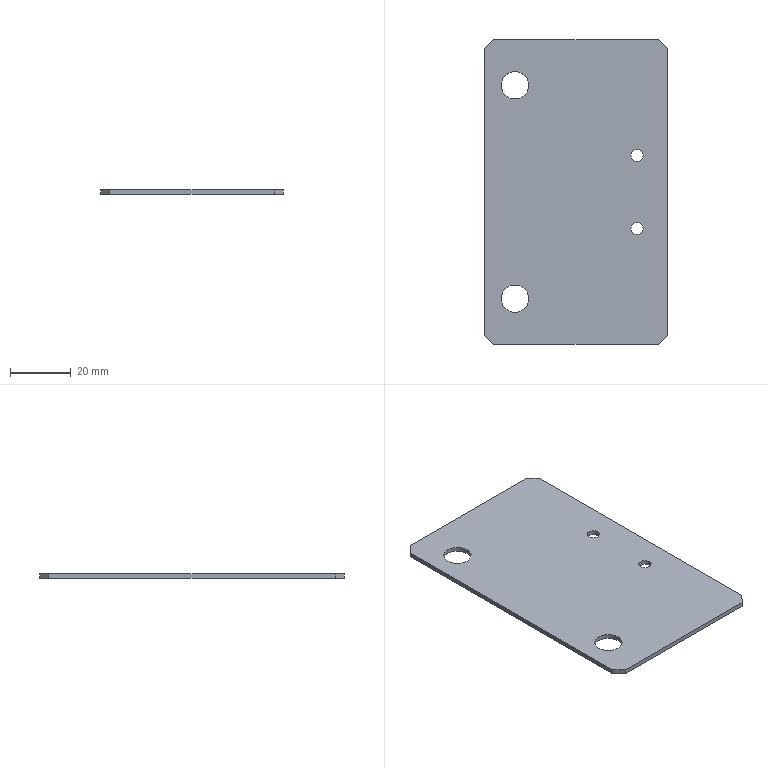Part | STEP file | 1 solid | 18 faces | box 60 x 100 x 1.5 mm | volume 8744 mm3 | plane 10 | cylinder 8 | commonest cylinder face diameters 4 x4 9 x4
STEP:
#1=CARTESIAN_POINT('',(0.,0.,0.));
#2=DIRECTION('',(0.,0.,1.));
#3=DIRECTION('',(1.,0.,0.));
#4=AXIS2_PLACEMENT_3D('',#1,#2,#3);
#5=CARTESIAN_POINT('',(-15.5,-35.,-1.5));
#6=VERTEX_POINT('',#5);
#7=CARTESIAN_POINT('',(-15.5,-35.,0.));
#8=VERTEX_POINT('',#7);
#9=CARTESIAN_POINT('',(-15.5,-35.,-1.5));
#10=DIRECTION('',(0.,0.,1.));
#11=VECTOR('',#10,1.);
#12=LINE('',#9,#11);
#13=CARTESIAN_POINT('',(-20.,-35.,-1.5));
#14=DIRECTION('',(0.,0.,1.));
#15=DIRECTION('',(1.,0.,0.));
#16=AXIS2_PLACEMENT_3D('',#13,#14,#15);
#17=CYLINDRICAL_SURFACE('',#16,4.5);
#18=CARTESIAN_POINT('',(6.283,0.));
#19=DIRECTION('',(0.,1.));
#20=VECTOR('',#19,1.);
#21=LINE('',#18,#20);
#22=(GEOMETRIC_REPRESENTATION_CONTEXT(2)PARAMETRIC_REPRESENTATION_CONTEXT()REPRESENTATION_CONTEXT('',''));
#23=DEFINITIONAL_REPRESENTATION('',(#21),#22);
#24=PCURVE('',#17,#23);
#25=CARTESIAN_POINT('',(-20.,-35.,-1.5));
#26=DIRECTION('',(0.,0.,1.));
#27=DIRECTION('',(1.,0.,0.));
#28=AXIS2_PLACEMENT_3D('',#25,#26,#27);
#29=CYLINDRICAL_SURFACE('',#28,4.5);
#30=CARTESIAN_POINT('',(0.,0.));
#31=DIRECTION('',(0.,1.));
#32=VECTOR('',#31,1.);
#33=LINE('',#30,#32);
#34=(GEOMETRIC_REPRESENTATION_CONTEXT(2)PARAMETRIC_REPRESENTATION_CONTEXT()REPRESENTATION_CONTEXT('',''));
#35=DEFINITIONAL_REPRESENTATION('',(#33),#34);
#36=PCURVE('',#29,#35);
#37=SURFACE_CURVE('',#12,(#24,#36),.PCURVE_S1.);
#38=EDGE_CURVE('',#6,#8,#37,.T.);
#39=ORIENTED_EDGE('',*,*,#38,.T.);
#40=CARTESIAN_POINT('',(-24.5,-35.,0.));
#41=VERTEX_POINT('',#40);
#42=CARTESIAN_POINT('',(-20.,-35.,0.));
#43=DIRECTION('',(0.,0.,1.));
#44=DIRECTION('',(1.,0.,0.));
#45=AXIS2_PLACEMENT_3D('',#42,#43,#44);
#46=CIRCLE('',#45,4.5);
#47=CARTESIAN_POINT('',(0.,1.5));
#48=DIRECTION('',(1.,0.));
#49=VECTOR('',#48,1.);
#50=LINE('',#47,#49);
#51=(GEOMETRIC_REPRESENTATION_CONTEXT(2)PARAMETRIC_REPRESENTATION_CONTEXT()REPRESENTATION_CONTEXT('',''));
#52=DEFINITIONAL_REPRESENTATION('',(#50),#51);
#53=PCURVE('',#17,#52);
#54=CARTESIAN_POINT('',(0.,0.,0.));
#55=DIRECTION('',(0.,0.,1.));
#56=DIRECTION('',(1.,0.,0.));
#57=AXIS2_PLACEMENT_3D('',#54,#55,#56);
#58=PLANE('',#57);
#59=CARTESIAN_POINT('',(-20.,-35.));
#60=DIRECTION('',(1.,0.));
#61=AXIS2_PLACEMENT_2D('',#59,#60);
#62=CIRCLE('',#61,4.5);
#63=(GEOMETRIC_REPRESENTATION_CONTEXT(2)PARAMETRIC_REPRESENTATION_CONTEXT()REPRESENTATION_CONTEXT('',''));
#64=DEFINITIONAL_REPRESENTATION('',(#62),#63);
#65=PCURVE('',#58,#64);
#66=SURFACE_CURVE('',#46,(#53,#65),.PCURVE_S1.);
#67=EDGE_CURVE('',#41,#8,#66,.T.);
#68=ORIENTED_EDGE('',*,*,#67,.F.);
#69=CARTESIAN_POINT('',(-24.5,-35.,-1.5));
#70=VERTEX_POINT('',#69);
#71=CARTESIAN_POINT('',(-24.5,-35.,-1.5));
#72=DIRECTION('',(0.,0.,1.));
#73=VECTOR('',#72,1.);
#74=LINE('',#71,#73);
#75=CARTESIAN_POINT('',(3.142,0.));
#76=DIRECTION('',(0.,1.));
#77=VECTOR('',#76,1.);
#78=LINE('',#75,#77);
#79=(GEOMETRIC_REPRESENTATION_CONTEXT(2)PARAMETRIC_REPRESENTATION_CONTEXT()REPRESENTATION_CONTEXT('',''));
#80=DEFINITIONAL_REPRESENTATION('',(#78),#79);
#81=PCURVE('',#17,#80);
#82=CARTESIAN_POINT('',(3.142,0.));
#83=DIRECTION('',(0.,1.));
#84=VECTOR('',#83,1.);
#85=LINE('',#82,#84);
#86=(GEOMETRIC_REPRESENTATION_CONTEXT(2)PARAMETRIC_REPRESENTATION_CONTEXT()REPRESENTATION_CONTEXT('',''));
#87=DEFINITIONAL_REPRESENTATION('',(#85),#86);
#88=PCURVE('',#29,#87);
#89=SURFACE_CURVE('',#74,(#81,#88),.PCURVE_S1.);
#90=EDGE_CURVE('',#70,#41,#89,.T.);
#91=ORIENTED_EDGE('',*,*,#90,.F.);
#92=CARTESIAN_POINT('',(-20.,-35.,-1.5));
#93=DIRECTION('',(0.,0.,1.));
#94=DIRECTION('',(1.,0.,0.));
#95=AXIS2_PLACEMENT_3D('',#92,#93,#94);
#96=CIRCLE('',#95,4.5);
#97=CARTESIAN_POINT('',(0.,0.));
#98=DIRECTION('',(1.,0.));
#99=VECTOR('',#98,1.);
#100=LINE('',#97,#99);
#101=(GEOMETRIC_REPRESENTATION_CONTEXT(2)PARAMETRIC_REPRESENTATION_CONTEXT()REPRESENTATION_CONTEXT('',''));
#102=DEFINITIONAL_REPRESENTATION('',(#100),#101);
#103=PCURVE('',#17,#102);
#104=CARTESIAN_POINT('',(0.,0.,-1.5));
#105=DIRECTION('',(0.,0.,1.));
#106=DIRECTION('',(1.,0.,0.));
#107=AXIS2_PLACEMENT_3D('',#104,#105,#106);
#108=PLANE('',#107);
#109=CARTESIAN_POINT('',(-20.,-35.));
#110=DIRECTION('',(1.,0.));
#111=AXIS2_PLACEMENT_2D('',#109,#110);
#112=CIRCLE('',#111,4.5);
#113=(GEOMETRIC_REPRESENTATION_CONTEXT(2)PARAMETRIC_REPRESENTATION_CONTEXT()REPRESENTATION_CONTEXT('',''));
#114=DEFINITIONAL_REPRESENTATION('',(#112),#113);
#115=PCURVE('',#108,#114);
#116=SURFACE_CURVE('',#96,(#103,#115),.PCURVE_S1.);
#117=EDGE_CURVE('',#70,#6,#116,.T.);
#118=ORIENTED_EDGE('',*,*,#117,.T.);
#119=EDGE_LOOP('',(#39,#68,#91,#118));
#120=FACE_BOUND('',#119,.F.);
#121=ADVANCED_FACE('',(#120),#17,.F.);
#122=CARTESIAN_POINT('',(-15.5,35.,-1.5));
#123=VERTEX_POINT('',#122);
#124=CARTESIAN_POINT('',(-15.5,35.,0.));
#125=VERTEX_POINT('',#124);
#126=CARTESIAN_POINT('',(-15.5,35.,-1.5));
#127=DIRECTION('',(0.,0.,1.));
#128=VECTOR('',#127,1.);
#129=LINE('',#126,#128);
#130=CARTESIAN_POINT('',(-20.,35.,-1.5));
#131=DIRECTION('',(0.,0.,1.));
#132=DIRECTION('',(1.,0.,0.));
#133=AXIS2_PLACEMENT_3D('',#130,#131,#132);
#134=CYLINDRICAL_SURFACE('',#133,4.5);
#135=CARTESIAN_POINT('',(6.283,0.));
#136=DIRECTION('',(0.,1.));
#137=VECTOR('',#136,1.);
#138=LINE('',#135,#137);
#139=(GEOMETRIC_REPRESENTATION_CONTEXT(2)PARAMETRIC_REPRESENTATION_CONTEXT()REPRESENTATION_CONTEXT('',''));
#140=DEFINITIONAL_REPRESENTATION('',(#138),#139);
#141=PCURVE('',#134,#140);
#142=CARTESIAN_POINT('',(-20.,35.,-1.5));
#143=DIRECTION('',(0.,0.,1.));
#144=DIRECTION('',(1.,0.,0.));
#145=AXIS2_PLACEMENT_3D('',#142,#143,#144);
#146=CYLINDRICAL_SURFACE('',#145,4.5);
#147=CARTESIAN_POINT('',(0.,0.));
#148=DIRECTION('',(0.,1.));
#149=VECTOR('',#148,1.);
#150=LINE('',#147,#149);
#151=(GEOMETRIC_REPRESENTATION_CONTEXT(2)PARAMETRIC_REPRESENTATION_CONTEXT()REPRESENTATION_CONTEXT('',''));
#152=DEFINITIONAL_REPRESENTATION('',(#150),#151);
#153=PCURVE('',#146,#152);
#154=SURFACE_CURVE('',#129,(#141,#153),.PCURVE_S1.);
#155=EDGE_CURVE('',#123,#125,#154,.T.);
#156=ORIENTED_EDGE('',*,*,#155,.T.);
#157=CARTESIAN_POINT('',(-24.5,35.,0.));
#158=VERTEX_POINT('',#157);
#159=CARTESIAN_POINT('',(-20.,35.,0.));
#160=DIRECTION('',(0.,0.,1.));
#161=DIRECTION('',(1.,0.,0.));
#162=AXIS2_PLACEMENT_3D('',#159,#160,#161);
#163=CIRCLE('',#162,4.5);
#164=CARTESIAN_POINT('',(0.,1.5));
#165=DIRECTION('',(1.,0.));
#166=VECTOR('',#165,1.);
#167=LINE('',#164,#166);
#168=(GEOMETRIC_REPRESENTATION_CONTEXT(2)PARAMETRIC_REPRESENTATION_CONTEXT()REPRESENTATION_CONTEXT('',''));
#169=DEFINITIONAL_REPRESENTATION('',(#167),#168);
#170=PCURVE('',#134,#169);
#171=CARTESIAN_POINT('',(-20.,35.));
#172=DIRECTION('',(1.,0.));
#173=AXIS2_PLACEMENT_2D('',#171,#172);
#174=CIRCLE('',#173,4.5);
#175=(GEOMETRIC_REPRESENTATION_CONTEXT(2)PARAMETRIC_REPRESENTATION_CONTEXT()REPRESENTATION_CONTEXT('',''));
#176=DEFINITIONAL_REPRESENTATION('',(#174),#175);
#177=PCURVE('',#58,#176);
#178=SURFACE_CURVE('',#163,(#170,#177),.PCURVE_S1.);
#179=EDGE_CURVE('',#158,#125,#178,.T.);
#180=ORIENTED_EDGE('',*,*,#179,.F.);
#181=CARTESIAN_POINT('',(-24.5,35.,-1.5));
#182=VERTEX_POINT('',#181);
#183=CARTESIAN_POINT('',(-24.5,35.,-1.5));
#184=DIRECTION('',(0.,0.,1.));
#185=VECTOR('',#184,1.);
#186=LINE('',#183,#185);
#187=CARTESIAN_POINT('',(3.142,0.));
#188=DIRECTION('',(0.,1.));
#189=VECTOR('',#188,1.);
#190=LINE('',#187,#189);
#191=(GEOMETRIC_REPRESENTATION_CONTEXT(2)PARAMETRIC_REPRESENTATION_CONTEXT()REPRESENTATION_CONTEXT('',''));
#192=DEFINITIONAL_REPRESENTATION('',(#190),#191);
#193=PCURVE('',#134,#192);
#194=CARTESIAN_POINT('',(3.142,0.));
#195=DIRECTION('',(0.,1.));
#196=VECTOR('',#195,1.);
#197=LINE('',#194,#196);
#198=(GEOMETRIC_REPRESENTATION_CONTEXT(2)PARAMETRIC_REPRESENTATION_CONTEXT()REPRESENTATION_CONTEXT('',''));
#199=DEFINITIONAL_REPRESENTATION('',(#197),#198);
#200=PCURVE('',#146,#199);
#201=SURFACE_CURVE('',#186,(#193,#200),.PCURVE_S1.);
#202=EDGE_CURVE('',#182,#158,#201,.T.);
#203=ORIENTED_EDGE('',*,*,#202,.F.);
#204=CARTESIAN_POINT('',(-20.,35.,-1.5));
#205=DIRECTION('',(0.,0.,1.));
#206=DIRECTION('',(1.,0.,0.));
#207=AXIS2_PLACEMENT_3D('',#204,#205,#206);
#208=CIRCLE('',#207,4.5);
#209=CARTESIAN_POINT('',(0.,0.));
#210=DIRECTION('',(1.,0.));
#211=VECTOR('',#210,1.);
#212=LINE('',#209,#211);
#213=(GEOMETRIC_REPRESENTATION_CONTEXT(2)PARAMETRIC_REPRESENTATION_CONTEXT()REPRESENTATION_CONTEXT('',''));
#214=DEFINITIONAL_REPRESENTATION('',(#212),#213);
#215=PCURVE('',#134,#214);
#216=CARTESIAN_POINT('',(-20.,35.));
#217=DIRECTION('',(1.,0.));
#218=AXIS2_PLACEMENT_2D('',#216,#217);
#219=CIRCLE('',#218,4.5);
#220=(GEOMETRIC_REPRESENTATION_CONTEXT(2)PARAMETRIC_REPRESENTATION_CONTEXT()REPRESENTATION_CONTEXT('',''));
#221=DEFINITIONAL_REPRESENTATION('',(#219),#220);
#222=PCURVE('',#108,#221);
#223=SURFACE_CURVE('',#208,(#215,#222),.PCURVE_S1.);
#224=EDGE_CURVE('',#182,#123,#223,.T.);
#225=ORIENTED_EDGE('',*,*,#224,.T.);
#226=EDGE_LOOP('',(#156,#180,#203,#225));
#227=FACE_BOUND('',#226,.F.);
#228=ADVANCED_FACE('',(#227),#134,.F.);
#229=CARTESIAN_POINT('',(22.,-12.,-1.5));
#230=VERTEX_POINT('',#229);
#231=CARTESIAN_POINT('',(22.,-12.,0.));
#232=VERTEX_POINT('',#231);
#233=CARTESIAN_POINT('',(22.,-12.,-1.5));
#234=DIRECTION('',(0.,0.,1.));
#235=VECTOR('',#234,1.);
#236=LINE('',#233,#235);
#237=CARTESIAN_POINT('',(20.,-12.,-1.5));
#238=DIRECTION('',(0.,0.,1.));
#239=DIRECTION('',(1.,0.,0.));
#240=AXIS2_PLACEMENT_3D('',#237,#238,#239);
#241=CYLINDRICAL_SURFACE('',#240,2.);
#242=CARTESIAN_POINT('',(6.283,0.));
#243=DIRECTION('',(0.,1.));
#244=VECTOR('',#243,1.);
#245=LINE('',#242,#244);
#246=(GEOMETRIC_REPRESENTATION_CONTEXT(2)PARAMETRIC_REPRESENTATION_CONTEXT()REPRESENTATION_CONTEXT('',''));
#247=DEFINITIONAL_REPRESENTATION('',(#245),#246);
#248=PCURVE('',#241,#247);
#249=CARTESIAN_POINT('',(20.,-12.,-1.5));
#250=DIRECTION('',(0.,0.,1.));
#251=DIRECTION('',(1.,0.,0.));
#252=AXIS2_PLACEMENT_3D('',#249,#250,#251);
#253=CYLINDRICAL_SURFACE('',#252,2.);
#254=CARTESIAN_POINT('',(0.,0.));
#255=DIRECTION('',(0.,1.));
#256=VECTOR('',#255,1.);
#257=LINE('',#254,#256);
#258=(GEOMETRIC_REPRESENTATION_CONTEXT(2)PARAMETRIC_REPRESENTATION_CONTEXT()REPRESENTATION_CONTEXT('',''));
#259=DEFINITIONAL_REPRESENTATION('',(#257),#258);
#260=PCURVE('',#253,#259);
#261=SURFACE_CURVE('',#236,(#248,#260),.PCURVE_S1.);
#262=EDGE_CURVE('',#230,#232,#261,.T.);
#263=ORIENTED_EDGE('',*,*,#262,.T.);
#264=CARTESIAN_POINT('',(18.,-12.,0.));
#265=VERTEX_POINT('',#264);
#266=CARTESIAN_POINT('',(20.,-12.,0.));
#267=DIRECTION('',(0.,0.,1.));
#268=DIRECTION('',(1.,0.,0.));
#269=AXIS2_PLACEMENT_3D('',#266,#267,#268);
#270=CIRCLE('',#269,2.);
#271=CARTESIAN_POINT('',(0.,1.5));
#272=DIRECTION('',(1.,0.));
#273=VECTOR('',#272,1.);
#274=LINE('',#271,#273);
#275=(GEOMETRIC_REPRESENTATION_CONTEXT(2)PARAMETRIC_REPRESENTATION_CONTEXT()REPRESENTATION_CONTEXT('',''));
#276=DEFINITIONAL_REPRESENTATION('',(#274),#275);
#277=PCURVE('',#241,#276);
#278=CARTESIAN_POINT('',(20.,-12.));
#279=DIRECTION('',(1.,0.));
#280=AXIS2_PLACEMENT_2D('',#278,#279);
#281=CIRCLE('',#280,2.);
#282=(GEOMETRIC_REPRESENTATION_CONTEXT(2)PARAMETRIC_REPRESENTATION_CONTEXT()REPRESENTATION_CONTEXT('',''));
#283=DEFINITIONAL_REPRESENTATION('',(#281),#282);
#284=PCURVE('',#58,#283);
#285=SURFACE_CURVE('',#270,(#277,#284),.PCURVE_S1.);
#286=EDGE_CURVE('',#265,#232,#285,.T.);
#287=ORIENTED_EDGE('',*,*,#286,.F.);
#288=CARTESIAN_POINT('',(18.,-12.,-1.5));
#289=VERTEX_POINT('',#288);
#290=CARTESIAN_POINT('',(18.,-12.,-1.5));
#291=DIRECTION('',(0.,0.,1.));
#292=VECTOR('',#291,1.);
#293=LINE('',#290,#292);
#294=CARTESIAN_POINT('',(3.142,0.));
#295=DIRECTION('',(0.,1.));
#296=VECTOR('',#295,1.);
#297=LINE('',#294,#296);
#298=(GEOMETRIC_REPRESENTATION_CONTEXT(2)PARAMETRIC_REPRESENTATION_CONTEXT()REPRESENTATION_CONTEXT('',''));
#299=DEFINITIONAL_REPRESENTATION('',(#297),#298);
#300=PCURVE('',#241,#299);
#301=CARTESIAN_POINT('',(3.142,0.));
#302=DIRECTION('',(0.,1.));
#303=VECTOR('',#302,1.);
#304=LINE('',#301,#303);
#305=(GEOMETRIC_REPRESENTATION_CONTEXT(2)PARAMETRIC_REPRESENTATION_CONTEXT()REPRESENTATION_CONTEXT('',''));
#306=DEFINITIONAL_REPRESENTATION('',(#304),#305);
#307=PCURVE('',#253,#306);
#308=SURFACE_CURVE('',#293,(#300,#307),.PCURVE_S1.);
#309=EDGE_CURVE('',#289,#265,#308,.T.);
#310=ORIENTED_EDGE('',*,*,#309,.F.);
#311=CARTESIAN_POINT('',(20.,-12.,-1.5));
#312=DIRECTION('',(0.,0.,1.));
#313=DIRECTION('',(1.,0.,0.));
#314=AXIS2_PLACEMENT_3D('',#311,#312,#313);
#315=CIRCLE('',#314,2.);
#316=CARTESIAN_POINT('',(0.,0.));
#317=DIRECTION('',(1.,0.));
#318=VECTOR('',#317,1.);
#319=LINE('',#316,#318);
#320=(GEOMETRIC_REPRESENTATION_CONTEXT(2)PARAMETRIC_REPRESENTATION_CONTEXT()REPRESENTATION_CONTEXT('',''));
#321=DEFINITIONAL_REPRESENTATION('',(#319),#320);
#322=PCURVE('',#241,#321);
#323=CARTESIAN_POINT('',(20.,-12.));
#324=DIRECTION('',(1.,0.));
#325=AXIS2_PLACEMENT_2D('',#323,#324);
#326=CIRCLE('',#325,2.);
#327=(GEOMETRIC_REPRESENTATION_CONTEXT(2)PARAMETRIC_REPRESENTATION_CONTEXT()REPRESENTATION_CONTEXT('',''));
#328=DEFINITIONAL_REPRESENTATION('',(#326),#327);
#329=PCURVE('',#108,#328);
#330=SURFACE_CURVE('',#315,(#322,#329),.PCURVE_S1.);
#331=EDGE_CURVE('',#289,#230,#330,.T.);
#332=ORIENTED_EDGE('',*,*,#331,.T.);
#333=EDGE_LOOP('',(#263,#287,#310,#332));
#334=FACE_BOUND('',#333,.F.);
#335=ADVANCED_FACE('',(#334),#241,.F.);
#336=CARTESIAN_POINT('',(22.,12.,-1.5));
#337=VERTEX_POINT('',#336);
#338=CARTESIAN_POINT('',(22.,12.,0.));
#339=VERTEX_POINT('',#338);
#340=CARTESIAN_POINT('',(22.,12.,-1.5));
#341=DIRECTION('',(0.,0.,1.));
#342=VECTOR('',#341,1.);
#343=LINE('',#340,#342);
#344=CARTESIAN_POINT('',(20.,12.,-1.5));
#345=DIRECTION('',(0.,0.,1.));
#346=DIRECTION('',(1.,0.,0.));
#347=AXIS2_PLACEMENT_3D('',#344,#345,#346);
#348=CYLINDRICAL_SURFACE('',#347,2.);
#349=CARTESIAN_POINT('',(6.283,0.));
#350=DIRECTION('',(0.,1.));
#351=VECTOR('',#350,1.);
#352=LINE('',#349,#351);
#353=(GEOMETRIC_REPRESENTATION_CONTEXT(2)PARAMETRIC_REPRESENTATION_CONTEXT()REPRESENTATION_CONTEXT('',''));
#354=DEFINITIONAL_REPRESENTATION('',(#352),#353);
#355=PCURVE('',#348,#354);
#356=CARTESIAN_POINT('',(20.,12.,-1.5));
#357=DIRECTION('',(0.,0.,1.));
#358=DIRECTION('',(1.,0.,0.));
#359=AXIS2_PLACEMENT_3D('',#356,#357,#358);
#360=CYLINDRICAL_SURFACE('',#359,2.);
#361=CARTESIAN_POINT('',(0.,0.));
#362=DIRECTION('',(0.,1.));
#363=VECTOR('',#362,1.);
#364=LINE('',#361,#363);
#365=(GEOMETRIC_REPRESENTATION_CONTEXT(2)PARAMETRIC_REPRESENTATION_CONTEXT()REPRESENTATION_CONTEXT('',''));
#366=DEFINITIONAL_REPRESENTATION('',(#364),#365);
#367=PCURVE('',#360,#366);
#368=SURFACE_CURVE('',#343,(#355,#367),.PCURVE_S1.);
#369=EDGE_CURVE('',#337,#339,#368,.T.);
#370=ORIENTED_EDGE('',*,*,#369,.T.);
#371=CARTESIAN_POINT('',(18.,12.,0.));
#372=VERTEX_POINT('',#371);
#373=CARTESIAN_POINT('',(20.,12.,0.));
#374=DIRECTION('',(0.,0.,1.));
#375=DIRECTION('',(1.,0.,0.));
#376=AXIS2_PLACEMENT_3D('',#373,#374,#375);
#377=CIRCLE('',#376,2.);
#378=CARTESIAN_POINT('',(0.,1.5));
#379=DIRECTION('',(1.,0.));
#380=VECTOR('',#379,1.);
#381=LINE('',#378,#380);
#382=(GEOMETRIC_REPRESENTATION_CONTEXT(2)PARAMETRIC_REPRESENTATION_CONTEXT()REPRESENTATION_CONTEXT('',''));
#383=DEFINITIONAL_REPRESENTATION('',(#381),#382);
#384=PCURVE('',#348,#383);
#385=CARTESIAN_POINT('',(20.,12.));
#386=DIRECTION('',(1.,0.));
#387=AXIS2_PLACEMENT_2D('',#385,#386);
#388=CIRCLE('',#387,2.);
#389=(GEOMETRIC_REPRESENTATION_CONTEXT(2)PARAMETRIC_REPRESENTATION_CONTEXT()REPRESENTATION_CONTEXT('',''));
#390=DEFINITIONAL_REPRESENTATION('',(#388),#389);
#391=PCURVE('',#58,#390);
#392=SURFACE_CURVE('',#377,(#384,#391),.PCURVE_S1.);
#393=EDGE_CURVE('',#372,#339,#392,.T.);
#394=ORIENTED_EDGE('',*,*,#393,.F.);
#395=CARTESIAN_POINT('',(18.,12.,-1.5));
#396=VERTEX_POINT('',#395);
#397=CARTESIAN_POINT('',(18.,12.,-1.5));
#398=DIRECTION('',(0.,0.,1.));
#399=VECTOR('',#398,1.);
#400=LINE('',#397,#399);
#401=CARTESIAN_POINT('',(3.142,0.));
#402=DIRECTION('',(0.,1.));
#403=VECTOR('',#402,1.);
#404=LINE('',#401,#403);
#405=(GEOMETRIC_REPRESENTATION_CONTEXT(2)PARAMETRIC_REPRESENTATION_CONTEXT()REPRESENTATION_CONTEXT('',''));
#406=DEFINITIONAL_REPRESENTATION('',(#404),#405);
#407=PCURVE('',#348,#406);
#408=CARTESIAN_POINT('',(3.142,0.));
#409=DIRECTION('',(0.,1.));
#410=VECTOR('',#409,1.);
#411=LINE('',#408,#410);
#412=(GEOMETRIC_REPRESENTATION_CONTEXT(2)PARAMETRIC_REPRESENTATION_CONTEXT()REPRESENTATION_CONTEXT('',''));
#413=DEFINITIONAL_REPRESENTATION('',(#411),#412);
#414=PCURVE('',#360,#413);
#415=SURFACE_CURVE('',#400,(#407,#414),.PCURVE_S1.);
#416=EDGE_CURVE('',#396,#372,#415,.T.);
#417=ORIENTED_EDGE('',*,*,#416,.F.);
#418=CARTESIAN_POINT('',(20.,12.,-1.5));
#419=DIRECTION('',(0.,0.,1.));
#420=DIRECTION('',(1.,0.,0.));
#421=AXIS2_PLACEMENT_3D('',#418,#419,#420);
#422=CIRCLE('',#421,2.);
#423=CARTESIAN_POINT('',(0.,0.));
#424=DIRECTION('',(1.,0.));
#425=VECTOR('',#424,1.);
#426=LINE('',#423,#425);
#427=(GEOMETRIC_REPRESENTATION_CONTEXT(2)PARAMETRIC_REPRESENTATION_CONTEXT()REPRESENTATION_CONTEXT('',''));
#428=DEFINITIONAL_REPRESENTATION('',(#426),#427);
#429=PCURVE('',#348,#428);
#430=CARTESIAN_POINT('',(20.,12.));
#431=DIRECTION('',(1.,0.));
#432=AXIS2_PLACEMENT_2D('',#430,#431);
#433=CIRCLE('',#432,2.);
#434=(GEOMETRIC_REPRESENTATION_CONTEXT(2)PARAMETRIC_REPRESENTATION_CONTEXT()REPRESENTATION_CONTEXT('',''));
#435=DEFINITIONAL_REPRESENTATION('',(#433),#434);
#436=PCURVE('',#108,#435);
#437=SURFACE_CURVE('',#422,(#429,#436),.PCURVE_S1.);
#438=EDGE_CURVE('',#396,#337,#437,.T.);
#439=ORIENTED_EDGE('',*,*,#438,.T.);
#440=EDGE_LOOP('',(#370,#394,#417,#439));
#441=FACE_BOUND('',#440,.F.);
#442=ADVANCED_FACE('',(#441),#348,.F.);
#443=CARTESIAN_POINT('',(30.,-47.,0.));
#444=VERTEX_POINT('',#443);
#445=CARTESIAN_POINT('',(30.,47.,0.));
#446=VERTEX_POINT('',#445);
#447=CARTESIAN_POINT('',(30.,50.,0.));
#448=DIRECTION('',(0.,1.,0.));
#449=VECTOR('',#448,1.);
#450=LINE('',#447,#449);
#451=CARTESIAN_POINT('',(30.,50.,-1.5));
#452=DIRECTION('',(1.,0.,0.));
#453=DIRECTION('',(0.,1.,0.));
#454=AXIS2_PLACEMENT_3D('',#451,#452,#453);
#455=PLANE('',#454);
#456=CARTESIAN_POINT('',(0.,1.5));
#457=DIRECTION('',(1.,0.));
#458=VECTOR('',#457,1.);
#459=LINE('',#456,#458);
#460=(GEOMETRIC_REPRESENTATION_CONTEXT(2)PARAMETRIC_REPRESENTATION_CONTEXT()REPRESENTATION_CONTEXT('',''));
#461=DEFINITIONAL_REPRESENTATION('',(#459),#460);
#462=PCURVE('',#455,#461);
#463=CARTESIAN_POINT('',(30.,50.));
#464=DIRECTION('',(0.,1.));
#465=VECTOR('',#464,1.);
#466=LINE('',#463,#465);
#467=(GEOMETRIC_REPRESENTATION_CONTEXT(2)PARAMETRIC_REPRESENTATION_CONTEXT()REPRESENTATION_CONTEXT('',''));
#468=DEFINITIONAL_REPRESENTATION('',(#466),#467);
#469=PCURVE('',#58,#468);
#470=SURFACE_CURVE('',#450,(#462,#469),.PCURVE_S1.);
#471=EDGE_CURVE('',#444,#446,#470,.T.);
#472=ORIENTED_EDGE('',*,*,#471,.F.);
#473=CARTESIAN_POINT('',(30.,-47.,-1.5));
#474=VERTEX_POINT('',#473);
#475=CARTESIAN_POINT('',(30.,-47.,-1.5));
#476=DIRECTION('',(0.,0.,-1.));
#477=VECTOR('',#476,1.);
#478=LINE('',#475,#477);
#479=CARTESIAN_POINT('',(-97.,0.));
#480=DIRECTION('',(0.,-1.));
#481=VECTOR('',#480,1.);
#482=LINE('',#479,#481);
#483=(GEOMETRIC_REPRESENTATION_CONTEXT(2)PARAMETRIC_REPRESENTATION_CONTEXT()REPRESENTATION_CONTEXT('',''));
#484=DEFINITIONAL_REPRESENTATION('',(#482),#483);
#485=PCURVE('',#455,#484);
#486=CARTESIAN_POINT('',(27.,-50.,-1.5));
#487=DIRECTION('',(-0.7071,0.7071,0.));
#488=DIRECTION('',(0.,0.,1.));
#489=AXIS2_PLACEMENT_3D('',#486,#487,#488);
#490=PLANE('',#489);
#491=CARTESIAN_POINT('',(0.,4.243));
#492=DIRECTION('',(-1.,0.));
#493=VECTOR('',#492,1.);
#494=LINE('',#491,#493);
#495=(GEOMETRIC_REPRESENTATION_CONTEXT(2)PARAMETRIC_REPRESENTATION_CONTEXT()REPRESENTATION_CONTEXT('',''));
#496=DEFINITIONAL_REPRESENTATION('',(#494),#495);
#497=PCURVE('',#490,#496);
#498=SURFACE_CURVE('',#478,(#485,#497),.PCURVE_S1.);
#499=EDGE_CURVE('',#444,#474,#498,.T.);
#500=ORIENTED_EDGE('',*,*,#499,.T.);
#501=CARTESIAN_POINT('',(30.,47.,-1.5));
#502=VERTEX_POINT('',#501);
#503=CARTESIAN_POINT('',(30.,50.,-1.5));
#504=DIRECTION('',(0.,1.,0.));
#505=VECTOR('',#504,1.);
#506=LINE('',#503,#505);
#507=CARTESIAN_POINT('',(0.,0.));
#508=DIRECTION('',(1.,0.));
#509=VECTOR('',#508,1.);
#510=LINE('',#507,#509);
#511=(GEOMETRIC_REPRESENTATION_CONTEXT(2)PARAMETRIC_REPRESENTATION_CONTEXT()REPRESENTATION_CONTEXT('',''));
#512=DEFINITIONAL_REPRESENTATION('',(#510),#511);
#513=PCURVE('',#455,#512);
#514=CARTESIAN_POINT('',(30.,50.));
#515=DIRECTION('',(0.,1.));
#516=VECTOR('',#515,1.);
#517=LINE('',#514,#516);
#518=(GEOMETRIC_REPRESENTATION_CONTEXT(2)PARAMETRIC_REPRESENTATION_CONTEXT()REPRESENTATION_CONTEXT('',''));
#519=DEFINITIONAL_REPRESENTATION('',(#517),#518);
#520=PCURVE('',#108,#519);
#521=SURFACE_CURVE('',#506,(#513,#520),.PCURVE_S1.);
#522=EDGE_CURVE('',#474,#502,#521,.T.);
#523=ORIENTED_EDGE('',*,*,#522,.T.);
#524=CARTESIAN_POINT('',(30.,47.,-1.5));
#525=DIRECTION('',(0.,0.,1.));
#526=VECTOR('',#525,1.);
#527=LINE('',#524,#526);
#528=CARTESIAN_POINT('',(-3.,0.));
#529=DIRECTION('',(0.,1.));
#530=VECTOR('',#529,1.);
#531=LINE('',#528,#530);
#532=(GEOMETRIC_REPRESENTATION_CONTEXT(2)PARAMETRIC_REPRESENTATION_CONTEXT()REPRESENTATION_CONTEXT('',''));
#533=DEFINITIONAL_REPRESENTATION('',(#531),#532);
#534=PCURVE('',#455,#533);
#535=CARTESIAN_POINT('',(30.,47.,-1.5));
#536=DIRECTION('',(-0.7071,-0.7071,0.));
#537=DIRECTION('',(0.,0.,1.));
#538=AXIS2_PLACEMENT_3D('',#535,#536,#537);
#539=PLANE('',#538);
#540=CARTESIAN_POINT('',(0.,0.));
#541=DIRECTION('',(1.,0.));
#542=VECTOR('',#541,1.);
#543=LINE('',#540,#542);
#544=(GEOMETRIC_REPRESENTATION_CONTEXT(2)PARAMETRIC_REPRESENTATION_CONTEXT()REPRESENTATION_CONTEXT('',''));
#545=DEFINITIONAL_REPRESENTATION('',(#543),#544);
#546=PCURVE('',#539,#545);
#547=SURFACE_CURVE('',#527,(#534,#546),.PCURVE_S1.);
#548=EDGE_CURVE('',#502,#446,#547,.T.);
#549=ORIENTED_EDGE('',*,*,#548,.T.);
#550=EDGE_LOOP('',(#472,#500,#523,#549));
#551=FACE_BOUND('',#550,.T.);
#552=ADVANCED_FACE('',(#551),#455,.T.);
#553=CARTESIAN_POINT('',(-27.,-50.,0.));
#554=VERTEX_POINT('',#553);
#555=CARTESIAN_POINT('',(27.,-50.,0.));
#556=VERTEX_POINT('',#555);
#557=CARTESIAN_POINT('',(-30.,-50.,0.));
#558=DIRECTION('',(1.,0.,0.));
#559=VECTOR('',#558,1.);
#560=LINE('',#557,#559);
#561=CARTESIAN_POINT('',(-30.,-50.,-1.5));
#562=DIRECTION('',(0.,-1.,0.));
#563=DIRECTION('',(0.,0.,-1.));
#564=AXIS2_PLACEMENT_3D('',#561,#562,#563);
#565=PLANE('',#564);
#566=CARTESIAN_POINT('',(-1.5,0.));
#567=DIRECTION('',(0.,1.));
#568=VECTOR('',#567,1.);
#569=LINE('',#566,#568);
#570=(GEOMETRIC_REPRESENTATION_CONTEXT(2)PARAMETRIC_REPRESENTATION_CONTEXT()REPRESENTATION_CONTEXT('',''));
#571=DEFINITIONAL_REPRESENTATION('',(#569),#570);
#572=PCURVE('',#565,#571);
#573=CARTESIAN_POINT('',(-30.,-50.));
#574=DIRECTION('',(1.,0.));
#575=VECTOR('',#574,1.);
#576=LINE('',#573,#575);
#577=(GEOMETRIC_REPRESENTATION_CONTEXT(2)PARAMETRIC_REPRESENTATION_CONTEXT()REPRESENTATION_CONTEXT('',''));
#578=DEFINITIONAL_REPRESENTATION('',(#576),#577);
#579=PCURVE('',#58,#578);
#580=SURFACE_CURVE('',#560,(#572,#579),.PCURVE_S1.);
#581=EDGE_CURVE('',#554,#556,#580,.T.);
#582=ORIENTED_EDGE('',*,*,#581,.F.);
#583=CARTESIAN_POINT('',(-27.,-50.,-1.5));
#584=VERTEX_POINT('',#583);
#585=CARTESIAN_POINT('',(-27.,-50.,-1.5));
#586=DIRECTION('',(0.,0.,-1.));
#587=VECTOR('',#586,1.);
#588=LINE('',#585,#587);
#589=CARTESIAN_POINT('',(0.,3.));
#590=DIRECTION('',(1.,0.));
#591=VECTOR('',#590,1.);
#592=LINE('',#589,#591);
#593=(GEOMETRIC_REPRESENTATION_CONTEXT(2)PARAMETRIC_REPRESENTATION_CONTEXT()REPRESENTATION_CONTEXT('',''));
#594=DEFINITIONAL_REPRESENTATION('',(#592),#593);
#595=PCURVE('',#565,#594);
#596=CARTESIAN_POINT('',(-30.,-47.,-1.5));
#597=DIRECTION('',(0.7071,0.7071,0.));
#598=DIRECTION('',(0.,0.,1.));
#599=AXIS2_PLACEMENT_3D('',#596,#597,#598);
#600=PLANE('',#599);
#601=CARTESIAN_POINT('',(0.,4.243));
#602=DIRECTION('',(-1.,0.));
#603=VECTOR('',#602,1.);
#604=LINE('',#601,#603);
#605=(GEOMETRIC_REPRESENTATION_CONTEXT(2)PARAMETRIC_REPRESENTATION_CONTEXT()REPRESENTATION_CONTEXT('',''));
#606=DEFINITIONAL_REPRESENTATION('',(#604),#605);
#607=PCURVE('',#600,#606);
#608=SURFACE_CURVE('',#588,(#595,#607),.PCURVE_S1.);
#609=EDGE_CURVE('',#554,#584,#608,.T.);
#610=ORIENTED_EDGE('',*,*,#609,.T.);
#611=CARTESIAN_POINT('',(27.,-50.,-1.5));
#612=VERTEX_POINT('',#611);
#613=CARTESIAN_POINT('',(-30.,-50.,-1.5));
#614=DIRECTION('',(1.,0.,0.));
#615=VECTOR('',#614,1.);
#616=LINE('',#613,#615);
#617=CARTESIAN_POINT('',(0.,0.));
#618=DIRECTION('',(0.,1.));
#619=VECTOR('',#618,1.);
#620=LINE('',#617,#619);
#621=(GEOMETRIC_REPRESENTATION_CONTEXT(2)PARAMETRIC_REPRESENTATION_CONTEXT()REPRESENTATION_CONTEXT('',''));
#622=DEFINITIONAL_REPRESENTATION('',(#620),#621);
#623=PCURVE('',#565,#622);
#624=CARTESIAN_POINT('',(-30.,-50.));
#625=DIRECTION('',(1.,0.));
#626=VECTOR('',#625,1.);
#627=LINE('',#624,#626);
#628=(GEOMETRIC_REPRESENTATION_CONTEXT(2)PARAMETRIC_REPRESENTATION_CONTEXT()REPRESENTATION_CONTEXT('',''));
#629=DEFINITIONAL_REPRESENTATION('',(#627),#628);
#630=PCURVE('',#108,#629);
#631=SURFACE_CURVE('',#616,(#623,#630),.PCURVE_S1.);
#632=EDGE_CURVE('',#584,#612,#631,.T.);
#633=ORIENTED_EDGE('',*,*,#632,.T.);
#634=CARTESIAN_POINT('',(27.,-50.,-1.5));
#635=DIRECTION('',(0.,0.,1.));
#636=VECTOR('',#635,1.);
#637=LINE('',#634,#636);
#638=CARTESIAN_POINT('',(0.,57.));
#639=DIRECTION('',(-1.,0.));
#640=VECTOR('',#639,1.);
#641=LINE('',#638,#640);
#642=(GEOMETRIC_REPRESENTATION_CONTEXT(2)PARAMETRIC_REPRESENTATION_CONTEXT()REPRESENTATION_CONTEXT('',''));
#643=DEFINITIONAL_REPRESENTATION('',(#641),#642);
#644=PCURVE('',#565,#643);
#645=CARTESIAN_POINT('',(0.,0.));
#646=DIRECTION('',(1.,0.));
#647=VECTOR('',#646,1.);
#648=LINE('',#645,#647);
#649=(GEOMETRIC_REPRESENTATION_CONTEXT(2)PARAMETRIC_REPRESENTATION_CONTEXT()REPRESENTATION_CONTEXT('',''));
#650=DEFINITIONAL_REPRESENTATION('',(#648),#649);
#651=PCURVE('',#490,#650);
#652=SURFACE_CURVE('',#637,(#644,#651),.PCURVE_S1.);
#653=EDGE_CURVE('',#612,#556,#652,.T.);
#654=ORIENTED_EDGE('',*,*,#653,.T.);
#655=EDGE_LOOP('',(#582,#610,#633,#654));
#656=FACE_BOUND('',#655,.T.);
#657=ADVANCED_FACE('',(#656),#565,.T.);
#658=CARTESIAN_POINT('',(-30.,47.,-1.5));
#659=VERTEX_POINT('',#658);
#660=CARTESIAN_POINT('',(-30.,-47.,-1.5));
#661=VERTEX_POINT('',#660);
#662=CARTESIAN_POINT('',(-30.,50.,-1.5));
#663=DIRECTION('',(0.,-1.,0.));
#664=VECTOR('',#663,1.);
#665=LINE('',#662,#664);
#666=CARTESIAN_POINT('',(-30.,50.,-1.5));
#667=DIRECTION('',(-1.,0.,0.));
#668=DIRECTION('',(0.,-1.,0.));
#669=AXIS2_PLACEMENT_3D('',#666,#667,#668);
#670=PLANE('',#669);
#671=CARTESIAN_POINT('',(0.,0.));
#672=DIRECTION('',(1.,0.));
#673=VECTOR('',#672,1.);
#674=LINE('',#671,#673);
#675=(GEOMETRIC_REPRESENTATION_CONTEXT(2)PARAMETRIC_REPRESENTATION_CONTEXT()REPRESENTATION_CONTEXT('',''));
#676=DEFINITIONAL_REPRESENTATION('',(#674),#675);
#677=PCURVE('',#670,#676);
#678=CARTESIAN_POINT('',(-30.,50.));
#679=DIRECTION('',(0.,-1.));
#680=VECTOR('',#679,1.);
#681=LINE('',#678,#680);
#682=(GEOMETRIC_REPRESENTATION_CONTEXT(2)PARAMETRIC_REPRESENTATION_CONTEXT()REPRESENTATION_CONTEXT('',''));
#683=DEFINITIONAL_REPRESENTATION('',(#681),#682);
#684=PCURVE('',#108,#683);
#685=SURFACE_CURVE('',#665,(#677,#684),.PCURVE_S1.);
#686=EDGE_CURVE('',#659,#661,#685,.T.);
#687=ORIENTED_EDGE('',*,*,#686,.T.);
#688=CARTESIAN_POINT('',(-30.,-47.,0.));
#689=VERTEX_POINT('',#688);
#690=CARTESIAN_POINT('',(-30.,-47.,-1.5));
#691=DIRECTION('',(0.,0.,1.));
#692=VECTOR('',#691,1.);
#693=LINE('',#690,#692);
#694=CARTESIAN_POINT('',(97.,0.));
#695=DIRECTION('',(0.,1.));
#696=VECTOR('',#695,1.);
#697=LINE('',#694,#696);
#698=(GEOMETRIC_REPRESENTATION_CONTEXT(2)PARAMETRIC_REPRESENTATION_CONTEXT()REPRESENTATION_CONTEXT('',''));
#699=DEFINITIONAL_REPRESENTATION('',(#697),#698);
#700=PCURVE('',#670,#699);
#701=CARTESIAN_POINT('',(0.,0.));
#702=DIRECTION('',(1.,0.));
#703=VECTOR('',#702,1.);
#704=LINE('',#701,#703);
#705=(GEOMETRIC_REPRESENTATION_CONTEXT(2)PARAMETRIC_REPRESENTATION_CONTEXT()REPRESENTATION_CONTEXT('',''));
#706=DEFINITIONAL_REPRESENTATION('',(#704),#705);
#707=PCURVE('',#600,#706);
#708=SURFACE_CURVE('',#693,(#700,#707),.PCURVE_S1.);
#709=EDGE_CURVE('',#661,#689,#708,.T.);
#710=ORIENTED_EDGE('',*,*,#709,.T.);
#711=CARTESIAN_POINT('',(-30.,47.,0.));
#712=VERTEX_POINT('',#711);
#713=CARTESIAN_POINT('',(-30.,50.,0.));
#714=DIRECTION('',(0.,-1.,0.));
#715=VECTOR('',#714,1.);
#716=LINE('',#713,#715);
#717=CARTESIAN_POINT('',(0.,1.5));
#718=DIRECTION('',(1.,0.));
#719=VECTOR('',#718,1.);
#720=LINE('',#717,#719);
#721=(GEOMETRIC_REPRESENTATION_CONTEXT(2)PARAMETRIC_REPRESENTATION_CONTEXT()REPRESENTATION_CONTEXT('',''));
#722=DEFINITIONAL_REPRESENTATION('',(#720),#721);
#723=PCURVE('',#670,#722);
#724=CARTESIAN_POINT('',(-30.,50.));
#725=DIRECTION('',(0.,-1.));
#726=VECTOR('',#725,1.);
#727=LINE('',#724,#726);
#728=(GEOMETRIC_REPRESENTATION_CONTEXT(2)PARAMETRIC_REPRESENTATION_CONTEXT()REPRESENTATION_CONTEXT('',''));
#729=DEFINITIONAL_REPRESENTATION('',(#727),#728);
#730=PCURVE('',#58,#729);
#731=SURFACE_CURVE('',#716,(#723,#730),.PCURVE_S1.);
#732=EDGE_CURVE('',#712,#689,#731,.T.);
#733=ORIENTED_EDGE('',*,*,#732,.F.);
#734=CARTESIAN_POINT('',(-30.,47.,-1.5));
#735=DIRECTION('',(0.,0.,-1.));
#736=VECTOR('',#735,1.);
#737=LINE('',#734,#736);
#738=CARTESIAN_POINT('',(3.,0.));
#739=DIRECTION('',(0.,-1.));
#740=VECTOR('',#739,1.);
#741=LINE('',#738,#740);
#742=(GEOMETRIC_REPRESENTATION_CONTEXT(2)PARAMETRIC_REPRESENTATION_CONTEXT()REPRESENTATION_CONTEXT('',''));
#743=DEFINITIONAL_REPRESENTATION('',(#741),#742);
#744=PCURVE('',#670,#743);
#745=CARTESIAN_POINT('',(-27.,50.,-1.5));
#746=DIRECTION('',(0.7071,-0.7071,0.));
#747=DIRECTION('',(0.,0.,1.));
#748=AXIS2_PLACEMENT_3D('',#745,#746,#747);
#749=PLANE('',#748);
#750=CARTESIAN_POINT('',(0.,4.243));
#751=DIRECTION('',(-1.,0.));
#752=VECTOR('',#751,1.);
#753=LINE('',#750,#752);
#754=(GEOMETRIC_REPRESENTATION_CONTEXT(2)PARAMETRIC_REPRESENTATION_CONTEXT()REPRESENTATION_CONTEXT('',''));
#755=DEFINITIONAL_REPRESENTATION('',(#753),#754);
#756=PCURVE('',#749,#755);
#757=SURFACE_CURVE('',#737,(#744,#756),.PCURVE_S1.);
#758=EDGE_CURVE('',#712,#659,#757,.T.);
#759=ORIENTED_EDGE('',*,*,#758,.T.);
#760=EDGE_LOOP('',(#687,#710,#733,#759));
#761=FACE_BOUND('',#760,.T.);
#762=ADVANCED_FACE('',(#761),#670,.T.);
#763=CARTESIAN_POINT('',(27.,50.,0.));
#764=VERTEX_POINT('',#763);
#765=CARTESIAN_POINT('',(-27.,50.,0.));
#766=VERTEX_POINT('',#765);
#767=CARTESIAN_POINT('',(-30.,50.,0.));
#768=DIRECTION('',(-1.,0.,0.));
#769=VECTOR('',#768,1.);
#770=LINE('',#767,#769);
#771=CARTESIAN_POINT('',(-30.,50.,-1.5));
#772=DIRECTION('',(0.,1.,0.));
#773=DIRECTION('',(0.,0.,1.));
#774=AXIS2_PLACEMENT_3D('',#771,#772,#773);
#775=PLANE('',#774);
#776=CARTESIAN_POINT('',(1.5,0.));
#777=DIRECTION('',(0.,-1.));
#778=VECTOR('',#777,1.);
#779=LINE('',#776,#778);
#780=(GEOMETRIC_REPRESENTATION_CONTEXT(2)PARAMETRIC_REPRESENTATION_CONTEXT()REPRESENTATION_CONTEXT('',''));
#781=DEFINITIONAL_REPRESENTATION('',(#779),#780);
#782=PCURVE('',#775,#781);
#783=CARTESIAN_POINT('',(-30.,50.));
#784=DIRECTION('',(-1.,0.));
#785=VECTOR('',#784,1.);
#786=LINE('',#783,#785);
#787=(GEOMETRIC_REPRESENTATION_CONTEXT(2)PARAMETRIC_REPRESENTATION_CONTEXT()REPRESENTATION_CONTEXT('',''));
#788=DEFINITIONAL_REPRESENTATION('',(#786),#787);
#789=PCURVE('',#58,#788);
#790=SURFACE_CURVE('',#770,(#782,#789),.PCURVE_S1.);
#791=EDGE_CURVE('',#764,#766,#790,.T.);
#792=ORIENTED_EDGE('',*,*,#791,.F.);
#793=CARTESIAN_POINT('',(27.,50.,-1.5));
#794=VERTEX_POINT('',#793);
#795=CARTESIAN_POINT('',(27.,50.,-1.5));
#796=DIRECTION('',(0.,0.,-1.));
#797=VECTOR('',#796,1.);
#798=LINE('',#795,#797);
#799=CARTESIAN_POINT('',(0.,57.));
#800=DIRECTION('',(-1.,0.));
#801=VECTOR('',#800,1.);
#802=LINE('',#799,#801);
#803=(GEOMETRIC_REPRESENTATION_CONTEXT(2)PARAMETRIC_REPRESENTATION_CONTEXT()REPRESENTATION_CONTEXT('',''));
#804=DEFINITIONAL_REPRESENTATION('',(#802),#803);
#805=PCURVE('',#775,#804);
#806=CARTESIAN_POINT('',(0.,4.243));
#807=DIRECTION('',(-1.,0.));
#808=VECTOR('',#807,1.);
#809=LINE('',#806,#808);
#810=(GEOMETRIC_REPRESENTATION_CONTEXT(2)PARAMETRIC_REPRESENTATION_CONTEXT()REPRESENTATION_CONTEXT('',''));
#811=DEFINITIONAL_REPRESENTATION('',(#809),#810);
#812=PCURVE('',#539,#811);
#813=SURFACE_CURVE('',#798,(#805,#812),.PCURVE_S1.);
#814=EDGE_CURVE('',#764,#794,#813,.T.);
#815=ORIENTED_EDGE('',*,*,#814,.T.);
#816=CARTESIAN_POINT('',(-27.,50.,-1.5));
#817=VERTEX_POINT('',#816);
#818=CARTESIAN_POINT('',(-30.,50.,-1.5));
#819=DIRECTION('',(-1.,0.,0.));
#820=VECTOR('',#819,1.);
#821=LINE('',#818,#820);
#822=CARTESIAN_POINT('',(0.,0.));
#823=DIRECTION('',(0.,-1.));
#824=VECTOR('',#823,1.);
#825=LINE('',#822,#824);
#826=(GEOMETRIC_REPRESENTATION_CONTEXT(2)PARAMETRIC_REPRESENTATION_CONTEXT()REPRESENTATION_CONTEXT('',''));
#827=DEFINITIONAL_REPRESENTATION('',(#825),#826);
#828=PCURVE('',#775,#827);
#829=CARTESIAN_POINT('',(-30.,50.));
#830=DIRECTION('',(-1.,0.));
#831=VECTOR('',#830,1.);
#832=LINE('',#829,#831);
#833=(GEOMETRIC_REPRESENTATION_CONTEXT(2)PARAMETRIC_REPRESENTATION_CONTEXT()REPRESENTATION_CONTEXT('',''));
#834=DEFINITIONAL_REPRESENTATION('',(#832),#833);
#835=PCURVE('',#108,#834);
#836=SURFACE_CURVE('',#821,(#828,#835),.PCURVE_S1.);
#837=EDGE_CURVE('',#794,#817,#836,.T.);
#838=ORIENTED_EDGE('',*,*,#837,.T.);
#839=CARTESIAN_POINT('',(-27.,50.,-1.5));
#840=DIRECTION('',(0.,0.,1.));
#841=VECTOR('',#840,1.);
#842=LINE('',#839,#841);
#843=CARTESIAN_POINT('',(0.,3.));
#844=DIRECTION('',(1.,0.));
#845=VECTOR('',#844,1.);
#846=LINE('',#843,#845);
#847=(GEOMETRIC_REPRESENTATION_CONTEXT(2)PARAMETRIC_REPRESENTATION_CONTEXT()REPRESENTATION_CONTEXT('',''));
#848=DEFINITIONAL_REPRESENTATION('',(#846),#847);
#849=PCURVE('',#775,#848);
#850=CARTESIAN_POINT('',(0.,0.));
#851=DIRECTION('',(1.,0.));
#852=VECTOR('',#851,1.);
#853=LINE('',#850,#852);
#854=(GEOMETRIC_REPRESENTATION_CONTEXT(2)PARAMETRIC_REPRESENTATION_CONTEXT()REPRESENTATION_CONTEXT('',''));
#855=DEFINITIONAL_REPRESENTATION('',(#853),#854);
#856=PCURVE('',#749,#855);
#857=SURFACE_CURVE('',#842,(#849,#856),.PCURVE_S1.);
#858=EDGE_CURVE('',#817,#766,#857,.T.);
#859=ORIENTED_EDGE('',*,*,#858,.T.);
#860=EDGE_LOOP('',(#792,#815,#838,#859));
#861=FACE_BOUND('',#860,.T.);
#862=ADVANCED_FACE('',(#861),#775,.T.);
#863=CARTESIAN_POINT('',(-20.,-35.,-1.5));
#864=DIRECTION('',(0.,0.,1.));
#865=DIRECTION('',(1.,0.,0.));
#866=AXIS2_PLACEMENT_3D('',#863,#864,#865);
#867=CIRCLE('',#866,4.5);
#868=CARTESIAN_POINT('',(-20.,-35.));
#869=DIRECTION('',(1.,0.));
#870=AXIS2_PLACEMENT_2D('',#868,#869);
#871=CIRCLE('',#870,4.5);
#872=(GEOMETRIC_REPRESENTATION_CONTEXT(2)PARAMETRIC_REPRESENTATION_CONTEXT()REPRESENTATION_CONTEXT('',''));
#873=DEFINITIONAL_REPRESENTATION('',(#871),#872);
#874=PCURVE('',#108,#873);
#875=CARTESIAN_POINT('',(0.,0.));
#876=DIRECTION('',(1.,0.));
#877=VECTOR('',#876,1.);
#878=LINE('',#875,#877);
#879=(GEOMETRIC_REPRESENTATION_CONTEXT(2)PARAMETRIC_REPRESENTATION_CONTEXT()REPRESENTATION_CONTEXT('',''));
#880=DEFINITIONAL_REPRESENTATION('',(#878),#879);
#881=PCURVE('',#29,#880);
#882=SURFACE_CURVE('',#867,(#874,#881),.PCURVE_S1.);
#883=EDGE_CURVE('',#6,#70,#882,.T.);
#884=ORIENTED_EDGE('',*,*,#883,.T.);
#885=ORIENTED_EDGE('',*,*,#117,.T.);
#886=EDGE_LOOP('',(#884,#885));
#887=FACE_BOUND('',#886,.T.);
#888=CARTESIAN_POINT('',(-20.,35.,-1.5));
#889=DIRECTION('',(0.,0.,1.));
#890=DIRECTION('',(1.,0.,0.));
#891=AXIS2_PLACEMENT_3D('',#888,#889,#890);
#892=CIRCLE('',#891,4.5);
#893=CARTESIAN_POINT('',(-20.,35.));
#894=DIRECTION('',(1.,0.));
#895=AXIS2_PLACEMENT_2D('',#893,#894);
#896=CIRCLE('',#895,4.5);
#897=(GEOMETRIC_REPRESENTATION_CONTEXT(2)PARAMETRIC_REPRESENTATION_CONTEXT()REPRESENTATION_CONTEXT('',''));
#898=DEFINITIONAL_REPRESENTATION('',(#896),#897);
#899=PCURVE('',#108,#898);
#900=CARTESIAN_POINT('',(0.,0.));
#901=DIRECTION('',(1.,0.));
#902=VECTOR('',#901,1.);
#903=LINE('',#900,#902);
#904=(GEOMETRIC_REPRESENTATION_CONTEXT(2)PARAMETRIC_REPRESENTATION_CONTEXT()REPRESENTATION_CONTEXT('',''));
#905=DEFINITIONAL_REPRESENTATION('',(#903),#904);
#906=PCURVE('',#146,#905);
#907=SURFACE_CURVE('',#892,(#899,#906),.PCURVE_S1.);
#908=EDGE_CURVE('',#123,#182,#907,.T.);
#909=ORIENTED_EDGE('',*,*,#908,.T.);
#910=ORIENTED_EDGE('',*,*,#224,.T.);
#911=EDGE_LOOP('',(#909,#910));
#912=FACE_BOUND('',#911,.T.);
#913=CARTESIAN_POINT('',(20.,-12.,-1.5));
#914=DIRECTION('',(0.,0.,1.));
#915=DIRECTION('',(1.,0.,0.));
#916=AXIS2_PLACEMENT_3D('',#913,#914,#915);
#917=CIRCLE('',#916,2.);
#918=CARTESIAN_POINT('',(20.,-12.));
#919=DIRECTION('',(1.,0.));
#920=AXIS2_PLACEMENT_2D('',#918,#919);
#921=CIRCLE('',#920,2.);
#922=(GEOMETRIC_REPRESENTATION_CONTEXT(2)PARAMETRIC_REPRESENTATION_CONTEXT()REPRESENTATION_CONTEXT('',''));
#923=DEFINITIONAL_REPRESENTATION('',(#921),#922);
#924=PCURVE('',#108,#923);
#925=CARTESIAN_POINT('',(0.,0.));
#926=DIRECTION('',(1.,0.));
#927=VECTOR('',#926,1.);
#928=LINE('',#925,#927);
#929=(GEOMETRIC_REPRESENTATION_CONTEXT(2)PARAMETRIC_REPRESENTATION_CONTEXT()REPRESENTATION_CONTEXT('',''));
#930=DEFINITIONAL_REPRESENTATION('',(#928),#929);
#931=PCURVE('',#253,#930);
#932=SURFACE_CURVE('',#917,(#924,#931),.PCURVE_S1.);
#933=EDGE_CURVE('',#230,#289,#932,.T.);
#934=ORIENTED_EDGE('',*,*,#933,.T.);
#935=ORIENTED_EDGE('',*,*,#331,.T.);
#936=EDGE_LOOP('',(#934,#935));
#937=FACE_BOUND('',#936,.T.);
#938=CARTESIAN_POINT('',(20.,12.,-1.5));
#939=DIRECTION('',(0.,0.,1.));
#940=DIRECTION('',(1.,0.,0.));
#941=AXIS2_PLACEMENT_3D('',#938,#939,#940);
#942=CIRCLE('',#941,2.);
#943=CARTESIAN_POINT('',(20.,12.));
#944=DIRECTION('',(1.,0.));
#945=AXIS2_PLACEMENT_2D('',#943,#944);
#946=CIRCLE('',#945,2.);
#947=(GEOMETRIC_REPRESENTATION_CONTEXT(2)PARAMETRIC_REPRESENTATION_CONTEXT()REPRESENTATION_CONTEXT('',''));
#948=DEFINITIONAL_REPRESENTATION('',(#946),#947);
#949=PCURVE('',#108,#948);
#950=CARTESIAN_POINT('',(0.,0.));
#951=DIRECTION('',(1.,0.));
#952=VECTOR('',#951,1.);
#953=LINE('',#950,#952);
#954=(GEOMETRIC_REPRESENTATION_CONTEXT(2)PARAMETRIC_REPRESENTATION_CONTEXT()REPRESENTATION_CONTEXT('',''));
#955=DEFINITIONAL_REPRESENTATION('',(#953),#954);
#956=PCURVE('',#360,#955);
#957=SURFACE_CURVE('',#942,(#949,#956),.PCURVE_S1.);
#958=EDGE_CURVE('',#337,#396,#957,.T.);
#959=ORIENTED_EDGE('',*,*,#958,.T.);
#960=ORIENTED_EDGE('',*,*,#438,.T.);
#961=EDGE_LOOP('',(#959,#960));
#962=FACE_BOUND('',#961,.T.);
#963=ORIENTED_EDGE('',*,*,#632,.F.);
#964=CARTESIAN_POINT('',(-30.,-47.,-1.5));
#965=DIRECTION('',(-0.7071,0.7071,0.));
#966=VECTOR('',#965,1.);
#967=LINE('',#964,#966);
#968=CARTESIAN_POINT('',(-30.,-47.));
#969=DIRECTION('',(-0.7071,0.7071));
#970=VECTOR('',#969,1.);
#971=LINE('',#968,#970);
#972=(GEOMETRIC_REPRESENTATION_CONTEXT(2)PARAMETRIC_REPRESENTATION_CONTEXT()REPRESENTATION_CONTEXT('',''));
#973=DEFINITIONAL_REPRESENTATION('',(#971),#972);
#974=PCURVE('',#108,#973);
#975=CARTESIAN_POINT('',(0.,0.));
#976=DIRECTION('',(0.,-1.));
#977=VECTOR('',#976,1.);
#978=LINE('',#975,#977);
#979=(GEOMETRIC_REPRESENTATION_CONTEXT(2)PARAMETRIC_REPRESENTATION_CONTEXT()REPRESENTATION_CONTEXT('',''));
#980=DEFINITIONAL_REPRESENTATION('',(#978),#979);
#981=PCURVE('',#600,#980);
#982=SURFACE_CURVE('',#967,(#974,#981),.PCURVE_S1.);
#983=EDGE_CURVE('',#584,#661,#982,.T.);
#984=ORIENTED_EDGE('',*,*,#983,.T.);
#985=ORIENTED_EDGE('',*,*,#686,.F.);
#986=CARTESIAN_POINT('',(-27.,50.,-1.5));
#987=DIRECTION('',(0.7071,0.7071,0.));
#988=VECTOR('',#987,1.);
#989=LINE('',#986,#988);
#990=CARTESIAN_POINT('',(-27.,50.));
#991=DIRECTION('',(0.7071,0.7071));
#992=VECTOR('',#991,1.);
#993=LINE('',#990,#992);
#994=(GEOMETRIC_REPRESENTATION_CONTEXT(2)PARAMETRIC_REPRESENTATION_CONTEXT()REPRESENTATION_CONTEXT('',''));
#995=DEFINITIONAL_REPRESENTATION('',(#993),#994);
#996=PCURVE('',#108,#995);
#997=CARTESIAN_POINT('',(0.,0.));
#998=DIRECTION('',(0.,-1.));
#999=VECTOR('',#998,1.);
#1000=LINE('',#997,#999);
#1001=(GEOMETRIC_REPRESENTATION_CONTEXT(2)PARAMETRIC_REPRESENTATION_CONTEXT()REPRESENTATION_CONTEXT('',''));
#1002=DEFINITIONAL_REPRESENTATION('',(#1000),#1001);
#1003=PCURVE('',#749,#1002);
#1004=SURFACE_CURVE('',#989,(#996,#1003),.PCURVE_S1.);
#1005=EDGE_CURVE('',#659,#817,#1004,.T.);
#1006=ORIENTED_EDGE('',*,*,#1005,.T.);
#1007=ORIENTED_EDGE('',*,*,#837,.F.);
#1008=CARTESIAN_POINT('',(30.,47.,-1.5));
#1009=DIRECTION('',(0.7071,-0.7071,0.));
#1010=VECTOR('',#1009,1.);
#1011=LINE('',#1008,#1010);
#1012=CARTESIAN_POINT('',(30.,47.));
#1013=DIRECTION('',(0.7071,-0.7071));
#1014=VECTOR('',#1013,1.);
#1015=LINE('',#1012,#1014);
#1016=(GEOMETRIC_REPRESENTATION_CONTEXT(2)PARAMETRIC_REPRESENTATION_CONTEXT()REPRESENTATION_CONTEXT('',''));
#1017=DEFINITIONAL_REPRESENTATION('',(#1015),#1016);
#1018=PCURVE('',#108,#1017);
#1019=CARTESIAN_POINT('',(0.,0.));
#1020=DIRECTION('',(0.,-1.));
#1021=VECTOR('',#1020,1.);
#1022=LINE('',#1019,#1021);
#1023=(GEOMETRIC_REPRESENTATION_CONTEXT(2)PARAMETRIC_REPRESENTATION_CONTEXT()REPRESENTATION_CONTEXT('',''));
#1024=DEFINITIONAL_REPRESENTATION('',(#1022),#1023);
#1025=PCURVE('',#539,#1024);
#1026=SURFACE_CURVE('',#1011,(#1018,#1025),.PCURVE_S1.);
#1027=EDGE_CURVE('',#794,#502,#1026,.T.);
#1028=ORIENTED_EDGE('',*,*,#1027,.T.);
#1029=ORIENTED_EDGE('',*,*,#522,.F.);
#1030=CARTESIAN_POINT('',(27.,-50.,-1.5));
#1031=DIRECTION('',(-0.7071,-0.7071,0.));
#1032=VECTOR('',#1031,1.);
#1033=LINE('',#1030,#1032);
#1034=CARTESIAN_POINT('',(27.,-50.));
#1035=DIRECTION('',(-0.7071,-0.7071));
#1036=VECTOR('',#1035,1.);
#1037=LINE('',#1034,#1036);
#1038=(GEOMETRIC_REPRESENTATION_CONTEXT(2)PARAMETRIC_REPRESENTATION_CONTEXT()REPRESENTATION_CONTEXT('',''));
#1039=DEFINITIONAL_REPRESENTATION('',(#1037),#1038);
#1040=PCURVE('',#108,#1039);
#1041=CARTESIAN_POINT('',(0.,0.));
#1042=DIRECTION('',(0.,-1.));
#1043=VECTOR('',#1042,1.);
#1044=LINE('',#1041,#1043);
#1045=(GEOMETRIC_REPRESENTATION_CONTEXT(2)PARAMETRIC_REPRESENTATION_CONTEXT()REPRESENTATION_CONTEXT('',''));
#1046=DEFINITIONAL_REPRESENTATION('',(#1044),#1045);
#1047=PCURVE('',#490,#1046);
#1048=SURFACE_CURVE('',#1033,(#1040,#1047),.PCURVE_S1.);
#1049=EDGE_CURVE('',#474,#612,#1048,.T.);
#1050=ORIENTED_EDGE('',*,*,#1049,.T.);
#1051=EDGE_LOOP('',(#963,#984,#985,#1006,#1007,#1028,#1029,#1050));
#1052=FACE_BOUND('',#1051,.T.);
#1053=ADVANCED_FACE('',(#887,#912,#937,#962,#1052),#108,.F.);
#1054=CARTESIAN_POINT('',(-20.,-35.,0.));
#1055=DIRECTION('',(0.,0.,1.));
#1056=DIRECTION('',(1.,0.,0.));
#1057=AXIS2_PLACEMENT_3D('',#1054,#1055,#1056);
#1058=CIRCLE('',#1057,4.5);
#1059=CARTESIAN_POINT('',(-20.,-35.));
#1060=DIRECTION('',(1.,0.));
#1061=AXIS2_PLACEMENT_2D('',#1059,#1060);
#1062=CIRCLE('',#1061,4.5);
#1063=(GEOMETRIC_REPRESENTATION_CONTEXT(2)PARAMETRIC_REPRESENTATION_CONTEXT()REPRESENTATION_CONTEXT('',''));
#1064=DEFINITIONAL_REPRESENTATION('',(#1062),#1063);
#1065=PCURVE('',#58,#1064);
#1066=CARTESIAN_POINT('',(0.,1.5));
#1067=DIRECTION('',(1.,0.));
#1068=VECTOR('',#1067,1.);
#1069=LINE('',#1066,#1068);
#1070=(GEOMETRIC_REPRESENTATION_CONTEXT(2)PARAMETRIC_REPRESENTATION_CONTEXT()REPRESENTATION_CONTEXT('',''));
#1071=DEFINITIONAL_REPRESENTATION('',(#1069),#1070);
#1072=PCURVE('',#29,#1071);
#1073=SURFACE_CURVE('',#1058,(#1065,#1072),.PCURVE_S1.);
#1074=EDGE_CURVE('',#8,#41,#1073,.T.);
#1075=ORIENTED_EDGE('',*,*,#1074,.F.);
#1076=ORIENTED_EDGE('',*,*,#67,.F.);
#1077=EDGE_LOOP('',(#1075,#1076));
#1078=FACE_BOUND('',#1077,.T.);
#1079=CARTESIAN_POINT('',(-20.,35.,0.));
#1080=DIRECTION('',(0.,0.,1.));
#1081=DIRECTION('',(1.,0.,0.));
#1082=AXIS2_PLACEMENT_3D('',#1079,#1080,#1081);
#1083=CIRCLE('',#1082,4.5);
#1084=CARTESIAN_POINT('',(-20.,35.));
#1085=DIRECTION('',(1.,0.));
#1086=AXIS2_PLACEMENT_2D('',#1084,#1085);
#1087=CIRCLE('',#1086,4.5);
#1088=(GEOMETRIC_REPRESENTATION_CONTEXT(2)PARAMETRIC_REPRESENTATION_CONTEXT()REPRESENTATION_CONTEXT('',''));
#1089=DEFINITIONAL_REPRESENTATION('',(#1087),#1088);
#1090=PCURVE('',#58,#1089);
#1091=CARTESIAN_POINT('',(0.,1.5));
#1092=DIRECTION('',(1.,0.));
#1093=VECTOR('',#1092,1.);
#1094=LINE('',#1091,#1093);
#1095=(GEOMETRIC_REPRESENTATION_CONTEXT(2)PARAMETRIC_REPRESENTATION_CONTEXT()REPRESENTATION_CONTEXT('',''));
#1096=DEFINITIONAL_REPRESENTATION('',(#1094),#1095);
#1097=PCURVE('',#146,#1096);
#1098=SURFACE_CURVE('',#1083,(#1090,#1097),.PCURVE_S1.);
#1099=EDGE_CURVE('',#125,#158,#1098,.T.);
#1100=ORIENTED_EDGE('',*,*,#1099,.F.);
#1101=ORIENTED_EDGE('',*,*,#179,.F.);
#1102=EDGE_LOOP('',(#1100,#1101));
#1103=FACE_BOUND('',#1102,.T.);
#1104=CARTESIAN_POINT('',(20.,-12.,0.));
#1105=DIRECTION('',(0.,0.,1.));
#1106=DIRECTION('',(1.,0.,0.));
#1107=AXIS2_PLACEMENT_3D('',#1104,#1105,#1106);
#1108=CIRCLE('',#1107,2.);
#1109=CARTESIAN_POINT('',(20.,-12.));
#1110=DIRECTION('',(1.,0.));
#1111=AXIS2_PLACEMENT_2D('',#1109,#1110);
#1112=CIRCLE('',#1111,2.);
#1113=(GEOMETRIC_REPRESENTATION_CONTEXT(2)PARAMETRIC_REPRESENTATION_CONTEXT()REPRESENTATION_CONTEXT('',''));
#1114=DEFINITIONAL_REPRESENTATION('',(#1112),#1113);
#1115=PCURVE('',#58,#1114);
#1116=CARTESIAN_POINT('',(0.,1.5));
#1117=DIRECTION('',(1.,0.));
#1118=VECTOR('',#1117,1.);
#1119=LINE('',#1116,#1118);
#1120=(GEOMETRIC_REPRESENTATION_CONTEXT(2)PARAMETRIC_REPRESENTATION_CONTEXT()REPRESENTATION_CONTEXT('',''));
#1121=DEFINITIONAL_REPRESENTATION('',(#1119),#1120);
#1122=PCURVE('',#253,#1121);
#1123=SURFACE_CURVE('',#1108,(#1115,#1122),.PCURVE_S1.);
#1124=EDGE_CURVE('',#232,#265,#1123,.T.);
#1125=ORIENTED_EDGE('',*,*,#1124,.F.);
#1126=ORIENTED_EDGE('',*,*,#286,.F.);
#1127=EDGE_LOOP('',(#1125,#1126));
#1128=FACE_BOUND('',#1127,.T.);
#1129=CARTESIAN_POINT('',(20.,12.,0.));
#1130=DIRECTION('',(0.,0.,1.));
#1131=DIRECTION('',(1.,0.,0.));
#1132=AXIS2_PLACEMENT_3D('',#1129,#1130,#1131);
#1133=CIRCLE('',#1132,2.);
#1134=CARTESIAN_POINT('',(20.,12.));
#1135=DIRECTION('',(1.,0.));
#1136=AXIS2_PLACEMENT_2D('',#1134,#1135);
#1137=CIRCLE('',#1136,2.);
#1138=(GEOMETRIC_REPRESENTATION_CONTEXT(2)PARAMETRIC_REPRESENTATION_CONTEXT()REPRESENTATION_CONTEXT('',''));
#1139=DEFINITIONAL_REPRESENTATION('',(#1137),#1138);
#1140=PCURVE('',#58,#1139);
#1141=CARTESIAN_POINT('',(0.,1.5));
#1142=DIRECTION('',(1.,0.));
#1143=VECTOR('',#1142,1.);
#1144=LINE('',#1141,#1143);
#1145=(GEOMETRIC_REPRESENTATION_CONTEXT(2)PARAMETRIC_REPRESENTATION_CONTEXT()REPRESENTATION_CONTEXT('',''));
#1146=DEFINITIONAL_REPRESENTATION('',(#1144),#1145);
#1147=PCURVE('',#360,#1146);
#1148=SURFACE_CURVE('',#1133,(#1140,#1147),.PCURVE_S1.);
#1149=EDGE_CURVE('',#339,#372,#1148,.T.);
#1150=ORIENTED_EDGE('',*,*,#1149,.F.);
#1151=ORIENTED_EDGE('',*,*,#393,.F.);
#1152=EDGE_LOOP('',(#1150,#1151));
#1153=FACE_BOUND('',#1152,.T.);
#1154=ORIENTED_EDGE('',*,*,#732,.T.);
#1155=CARTESIAN_POINT('',(-38.5,-38.5,0.));
#1156=DIRECTION('',(0.7071,-0.7071,0.));
#1157=VECTOR('',#1156,1.);
#1158=LINE('',#1155,#1157);
#1159=CARTESIAN_POINT('',(-38.5,-38.5));
#1160=DIRECTION('',(0.7071,-0.7071));
#1161=VECTOR('',#1160,1.);
#1162=LINE('',#1159,#1161);
#1163=(GEOMETRIC_REPRESENTATION_CONTEXT(2)PARAMETRIC_REPRESENTATION_CONTEXT()REPRESENTATION_CONTEXT('',''));
#1164=DEFINITIONAL_REPRESENTATION('',(#1162),#1163);
#1165=PCURVE('',#58,#1164);
#1166=CARTESIAN_POINT('',(1.5,-12.021));
#1167=DIRECTION('',(0.,1.));
#1168=VECTOR('',#1167,1.);
#1169=LINE('',#1166,#1168);
#1170=(GEOMETRIC_REPRESENTATION_CONTEXT(2)PARAMETRIC_REPRESENTATION_CONTEXT()REPRESENTATION_CONTEXT('',''));
#1171=DEFINITIONAL_REPRESENTATION('',(#1169),#1170);
#1172=PCURVE('',#600,#1171);
#1173=SURFACE_CURVE('',#1158,(#1165,#1172),.PCURVE_S1.);
#1174=EDGE_CURVE('',#689,#554,#1173,.T.);
#1175=ORIENTED_EDGE('',*,*,#1174,.T.);
#1176=ORIENTED_EDGE('',*,*,#581,.T.);
#1177=CARTESIAN_POINT('',(38.5,-38.5,0.));
#1178=DIRECTION('',(0.7071,0.7071,0.));
#1179=VECTOR('',#1178,1.);
#1180=LINE('',#1177,#1179);
#1181=CARTESIAN_POINT('',(38.5,-38.5));
#1182=DIRECTION('',(0.7071,0.7071));
#1183=VECTOR('',#1182,1.);
#1184=LINE('',#1181,#1183);
#1185=(GEOMETRIC_REPRESENTATION_CONTEXT(2)PARAMETRIC_REPRESENTATION_CONTEXT()REPRESENTATION_CONTEXT('',''));
#1186=DEFINITIONAL_REPRESENTATION('',(#1184),#1185);
#1187=PCURVE('',#58,#1186);
#1188=CARTESIAN_POINT('',(1.5,16.263));
#1189=DIRECTION('',(0.,1.));
#1190=VECTOR('',#1189,1.);
#1191=LINE('',#1188,#1190);
#1192=(GEOMETRIC_REPRESENTATION_CONTEXT(2)PARAMETRIC_REPRESENTATION_CONTEXT()REPRESENTATION_CONTEXT('',''));
#1193=DEFINITIONAL_REPRESENTATION('',(#1191),#1192);
#1194=PCURVE('',#490,#1193);
#1195=SURFACE_CURVE('',#1180,(#1187,#1194),.PCURVE_S1.);
#1196=EDGE_CURVE('',#556,#444,#1195,.T.);
#1197=ORIENTED_EDGE('',*,*,#1196,.T.);
#1198=ORIENTED_EDGE('',*,*,#471,.T.);
#1199=CARTESIAN_POINT('',(38.5,38.5,0.));
#1200=DIRECTION('',(-0.7071,0.7071,0.));
#1201=VECTOR('',#1200,1.);
#1202=LINE('',#1199,#1201);
#1203=CARTESIAN_POINT('',(38.5,38.5));
#1204=DIRECTION('',(-0.7071,0.7071));
#1205=VECTOR('',#1204,1.);
#1206=LINE('',#1203,#1205);
#1207=(GEOMETRIC_REPRESENTATION_CONTEXT(2)PARAMETRIC_REPRESENTATION_CONTEXT()REPRESENTATION_CONTEXT('',''));
#1208=DEFINITIONAL_REPRESENTATION('',(#1206),#1207);
#1209=PCURVE('',#58,#1208);
#1210=CARTESIAN_POINT('',(1.5,-12.021));
#1211=DIRECTION('',(0.,1.));
#1212=VECTOR('',#1211,1.);
#1213=LINE('',#1210,#1212);
#1214=(GEOMETRIC_REPRESENTATION_CONTEXT(2)PARAMETRIC_REPRESENTATION_CONTEXT()REPRESENTATION_CONTEXT('',''));
#1215=DEFINITIONAL_REPRESENTATION('',(#1213),#1214);
#1216=PCURVE('',#539,#1215);
#1217=SURFACE_CURVE('',#1202,(#1209,#1216),.PCURVE_S1.);
#1218=EDGE_CURVE('',#446,#764,#1217,.T.);
#1219=ORIENTED_EDGE('',*,*,#1218,.T.);
#1220=ORIENTED_EDGE('',*,*,#791,.T.);
#1221=CARTESIAN_POINT('',(-38.5,38.5,0.));
#1222=DIRECTION('',(-0.7071,-0.7071,0.));
#1223=VECTOR('',#1222,1.);
#1224=LINE('',#1221,#1223);
#1225=CARTESIAN_POINT('',(-38.5,38.5));
#1226=DIRECTION('',(-0.7071,-0.7071));
#1227=VECTOR('',#1226,1.);
#1228=LINE('',#1225,#1227);
#1229=(GEOMETRIC_REPRESENTATION_CONTEXT(2)PARAMETRIC_REPRESENTATION_CONTEXT()REPRESENTATION_CONTEXT('',''));
#1230=DEFINITIONAL_REPRESENTATION('',(#1228),#1229);
#1231=PCURVE('',#58,#1230);
#1232=CARTESIAN_POINT('',(1.5,16.263));
#1233=DIRECTION('',(0.,1.));
#1234=VECTOR('',#1233,1.);
#1235=LINE('',#1232,#1234);
#1236=(GEOMETRIC_REPRESENTATION_CONTEXT(2)PARAMETRIC_REPRESENTATION_CONTEXT()REPRESENTATION_CONTEXT('',''));
#1237=DEFINITIONAL_REPRESENTATION('',(#1235),#1236);
#1238=PCURVE('',#749,#1237);
#1239=SURFACE_CURVE('',#1224,(#1231,#1238),.PCURVE_S1.);
#1240=EDGE_CURVE('',#766,#712,#1239,.T.);
#1241=ORIENTED_EDGE('',*,*,#1240,.T.);
#1242=EDGE_LOOP('',(#1154,#1175,#1176,#1197,#1198,#1219,#1220,#1241));
#1243=FACE_BOUND('',#1242,.T.);
#1244=ADVANCED_FACE('',(#1078,#1103,#1128,#1153,#1243),#58,.T.);
#1245=ORIENTED_EDGE('',*,*,#1149,.F.);
#1246=ORIENTED_EDGE('',*,*,#369,.F.);
#1247=ORIENTED_EDGE('',*,*,#958,.T.);
#1248=ORIENTED_EDGE('',*,*,#416,.T.);
#1249=EDGE_LOOP('',(#1245,#1246,#1247,#1248));
#1250=FACE_BOUND('',#1249,.F.);
#1251=ADVANCED_FACE('',(#1250),#360,.F.);
#1252=ORIENTED_EDGE('',*,*,#1124,.F.);
#1253=ORIENTED_EDGE('',*,*,#262,.F.);
#1254=ORIENTED_EDGE('',*,*,#933,.T.);
#1255=ORIENTED_EDGE('',*,*,#309,.T.);
#1256=EDGE_LOOP('',(#1252,#1253,#1254,#1255));
#1257=FACE_BOUND('',#1256,.F.);
#1258=ADVANCED_FACE('',(#1257),#253,.F.);
#1259=ORIENTED_EDGE('',*,*,#1099,.F.);
#1260=ORIENTED_EDGE('',*,*,#155,.F.);
#1261=ORIENTED_EDGE('',*,*,#908,.T.);
#1262=ORIENTED_EDGE('',*,*,#202,.T.);
#1263=EDGE_LOOP('',(#1259,#1260,#1261,#1262));
#1264=FACE_BOUND('',#1263,.F.);
#1265=ADVANCED_FACE('',(#1264),#146,.F.);
#1266=ORIENTED_EDGE('',*,*,#1074,.F.);
#1267=ORIENTED_EDGE('',*,*,#38,.F.);
#1268=ORIENTED_EDGE('',*,*,#883,.T.);
#1269=ORIENTED_EDGE('',*,*,#90,.T.);
#1270=EDGE_LOOP('',(#1266,#1267,#1268,#1269));
#1271=FACE_BOUND('',#1270,.F.);
#1272=ADVANCED_FACE('',(#1271),#29,.F.);
#1273=ORIENTED_EDGE('',*,*,#983,.F.);
#1274=ORIENTED_EDGE('',*,*,#609,.F.);
#1275=ORIENTED_EDGE('',*,*,#1174,.F.);
#1276=ORIENTED_EDGE('',*,*,#709,.F.);
#1277=EDGE_LOOP('',(#1273,#1274,#1275,#1276));
#1278=FACE_BOUND('',#1277,.T.);
#1279=ADVANCED_FACE('',(#1278),#600,.F.);
#1280=ORIENTED_EDGE('',*,*,#1049,.F.);
#1281=ORIENTED_EDGE('',*,*,#499,.F.);
#1282=ORIENTED_EDGE('',*,*,#1196,.F.);
#1283=ORIENTED_EDGE('',*,*,#653,.F.);
#1284=EDGE_LOOP('',(#1280,#1281,#1282,#1283));
#1285=FACE_BOUND('',#1284,.T.);
#1286=ADVANCED_FACE('',(#1285),#490,.F.);
#1287=ORIENTED_EDGE('',*,*,#1027,.F.);
#1288=ORIENTED_EDGE('',*,*,#814,.F.);
#1289=ORIENTED_EDGE('',*,*,#1218,.F.);
#1290=ORIENTED_EDGE('',*,*,#548,.F.);
#1291=EDGE_LOOP('',(#1287,#1288,#1289,#1290));
#1292=FACE_BOUND('',#1291,.T.);
#1293=ADVANCED_FACE('',(#1292),#539,.F.);
#1294=ORIENTED_EDGE('',*,*,#1005,.F.);
#1295=ORIENTED_EDGE('',*,*,#758,.F.);
#1296=ORIENTED_EDGE('',*,*,#1240,.F.);
#1297=ORIENTED_EDGE('',*,*,#858,.F.);
#1298=EDGE_LOOP('',(#1294,#1295,#1296,#1297));
#1299=FACE_BOUND('',#1298,.T.);
#1300=ADVANCED_FACE('',(#1299),#749,.F.);
#1301=CLOSED_SHELL('',(#121,#228,#335,#442,#552,#657,#762,#862,#1053,#1244,#1251,#1258,#1265,#1272,#1279,#1286,#1293,#1300));
#1302=MANIFOLD_SOLID_BREP('',#1301);
#1303=(LENGTH_UNIT()NAMED_UNIT(*)SI_UNIT(.MILLI.,.METRE.));
#1304=UNCERTAINTY_MEASURE_WITH_UNIT(LENGTH_MEASURE(0.0000001),#1303,'','');
#1305=(NAMED_UNIT(*)PLANE_ANGLE_UNIT()SI_UNIT($,.RADIAN.));
#1306=(NAMED_UNIT(*)SI_UNIT($,.STERADIAN.)SOLID_ANGLE_UNIT());
#1307=(GEOMETRIC_REPRESENTATION_CONTEXT(3)GLOBAL_UNCERTAINTY_ASSIGNED_CONTEXT((#1304))GLOBAL_UNIT_ASSIGNED_CONTEXT((#1303,#1305,#1306))REPRESENTATION_CONTEXT('',''));
#1308=ADVANCED_BREP_SHAPE_REPRESENTATION('',(#4,#1302),#1307);